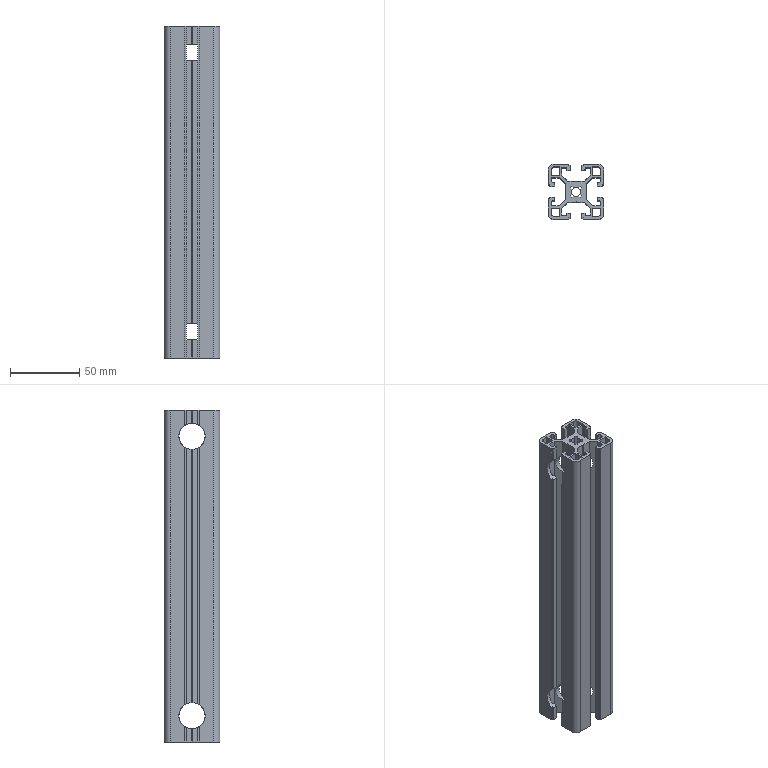Part | SolidWorks | features Extrusion 1, HoleWzd 1 | 1 solid | 273 faces | box 40 x 40 x 240 mm | volume 135882 mm3 | plane 213 | cylinder 60 | commonest cylinder face diameters 2 x16 6.8 x15 19 x12 1 x8 5 x4 9 x4